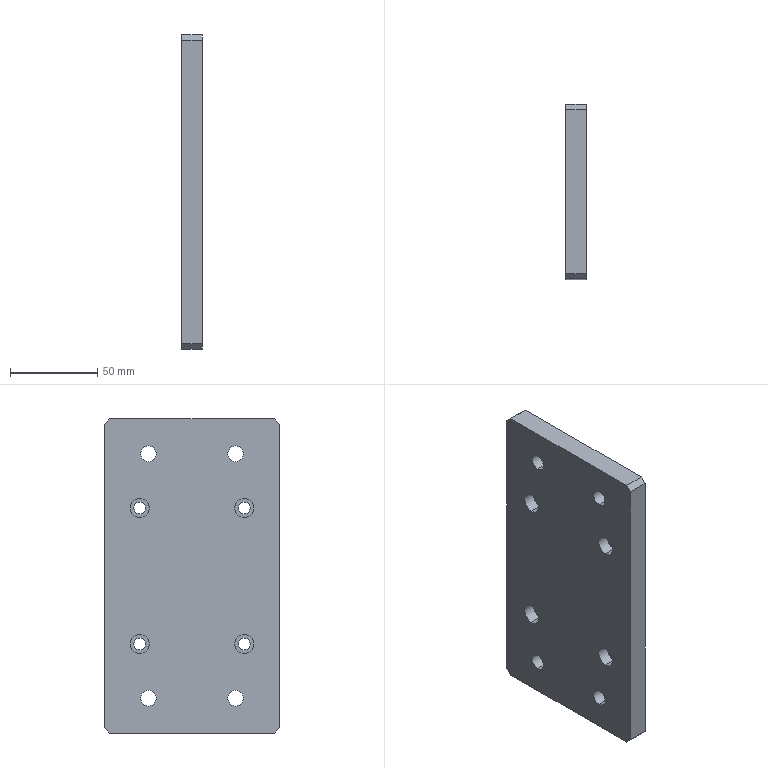Part | SolidWorks | features HoleWzd 2, Chamfer 1, Extrusion 1 | 1 solid | 38 faces | box 12 x 100 x 180 mm | volume 209434 mm3 | cylinder 24 | plane 14 | commonest cylinder face diameters 6.6 x8 9 x8 11 x8
STEP:
#1=CARTESIAN_POINT('',(12.,25.,-74.5));
#2=VERTEX_POINT('',#1);
#3=CARTESIAN_POINT('',(12.,25.,-65.5));
#4=VERTEX_POINT('',#3);
#5=CARTESIAN_POINT('',(12.,25.,-70.));
#6=DIRECTION('',(-1.,0.,0.));
#7=DIRECTION('',(0.,0.,1.));
#8=AXIS2_PLACEMENT_3D('',#5,#6,#7);
#9=CIRCLE('',#8,4.5);
#10=EDGE_CURVE('',#2,#4,#9,.T.);
#11=ORIENTED_EDGE('',*,*,#10,.F.);
#12=CARTESIAN_POINT('',(0.,25.,-74.5));
#13=VERTEX_POINT('',#12);
#14=CARTESIAN_POINT('',(0.,25.,-74.5));
#15=DIRECTION('',(-1.,0.,0.));
#16=VECTOR('',#15,1000.);
#17=LINE('',#14,#16);
#18=EDGE_CURVE('',#2,#13,#17,.T.);
#19=ORIENTED_EDGE('',*,*,#18,.T.);
#20=CARTESIAN_POINT('',(0.,25.,-65.5));
#21=VERTEX_POINT('',#20);
#22=CARTESIAN_POINT('',(0.,25.,-70.));
#23=DIRECTION('',(-1.,0.,0.));
#24=DIRECTION('',(0.,0.,1.));
#25=AXIS2_PLACEMENT_3D('',#22,#23,#24);
#26=CIRCLE('',#25,4.5);
#27=EDGE_CURVE('',#13,#21,#26,.T.);
#28=ORIENTED_EDGE('',*,*,#27,.T.);
#29=CARTESIAN_POINT('',(0.,25.,-65.5));
#30=DIRECTION('',(-1.,0.,0.));
#31=VECTOR('',#30,1000.);
#32=LINE('',#29,#31);
#33=EDGE_CURVE('',#4,#21,#32,.T.);
#34=ORIENTED_EDGE('',*,*,#33,.F.);
#35=EDGE_LOOP('',(#11,#19,#28,#34));
#36=FACE_OUTER_BOUND('',#35,.T.);
#37=CARTESIAN_POINT('',(0.,25.,-70.));
#38=DIRECTION('',(-1.,0.,0.));
#39=DIRECTION('',(0.,0.,1.));
#40=AXIS2_PLACEMENT_3D('',#37,#38,#39);
#41=CYLINDRICAL_SURFACE('',#40,4.5);
#42=ADVANCED_FACE('',(#36),#41,.F.);
#43=CARTESIAN_POINT('',(12.,-25.,-74.5));
#44=VERTEX_POINT('',#43);
#45=CARTESIAN_POINT('',(12.,-25.,-65.5));
#46=VERTEX_POINT('',#45);
#47=CARTESIAN_POINT('',(12.,-25.,-70.));
#48=DIRECTION('',(-1.,0.,0.));
#49=DIRECTION('',(0.,0.,1.));
#50=AXIS2_PLACEMENT_3D('',#47,#48,#49);
#51=CIRCLE('',#50,4.5);
#52=EDGE_CURVE('',#44,#46,#51,.T.);
#53=ORIENTED_EDGE('',*,*,#52,.F.);
#54=CARTESIAN_POINT('',(0.,-25.,-74.5));
#55=VERTEX_POINT('',#54);
#56=CARTESIAN_POINT('',(0.,-25.,-74.5));
#57=DIRECTION('',(-1.,0.,0.));
#58=VECTOR('',#57,1000.);
#59=LINE('',#56,#58);
#60=EDGE_CURVE('',#44,#55,#59,.T.);
#61=ORIENTED_EDGE('',*,*,#60,.T.);
#62=CARTESIAN_POINT('',(0.,-25.,-65.5));
#63=VERTEX_POINT('',#62);
#64=CARTESIAN_POINT('',(0.,-25.,-70.));
#65=DIRECTION('',(-1.,0.,0.));
#66=DIRECTION('',(0.,0.,1.));
#67=AXIS2_PLACEMENT_3D('',#64,#65,#66);
#68=CIRCLE('',#67,4.5);
#69=EDGE_CURVE('',#55,#63,#68,.T.);
#70=ORIENTED_EDGE('',*,*,#69,.T.);
#71=CARTESIAN_POINT('',(0.,-25.,-65.5));
#72=DIRECTION('',(-1.,0.,0.));
#73=VECTOR('',#72,1000.);
#74=LINE('',#71,#73);
#75=EDGE_CURVE('',#46,#63,#74,.T.);
#76=ORIENTED_EDGE('',*,*,#75,.F.);
#77=EDGE_LOOP('',(#53,#61,#70,#76));
#78=FACE_OUTER_BOUND('',#77,.T.);
#79=CARTESIAN_POINT('',(0.,-25.,-70.));
#80=DIRECTION('',(-1.,0.,0.));
#81=DIRECTION('',(0.,0.,1.));
#82=AXIS2_PLACEMENT_3D('',#79,#80,#81);
#83=CYLINDRICAL_SURFACE('',#82,4.5);
#84=ADVANCED_FACE('',(#78),#83,.F.);
#85=CARTESIAN_POINT('',(12.,25.,65.5));
#86=VERTEX_POINT('',#85);
#87=CARTESIAN_POINT('',(12.,25.,74.5));
#88=VERTEX_POINT('',#87);
#89=CARTESIAN_POINT('',(12.,25.,70.));
#90=DIRECTION('',(-1.,0.,0.));
#91=DIRECTION('',(0.,0.,1.));
#92=AXIS2_PLACEMENT_3D('',#89,#90,#91);
#93=CIRCLE('',#92,4.5);
#94=EDGE_CURVE('',#86,#88,#93,.T.);
#95=ORIENTED_EDGE('',*,*,#94,.F.);
#96=CARTESIAN_POINT('',(0.,25.,65.5));
#97=VERTEX_POINT('',#96);
#98=CARTESIAN_POINT('',(0.,25.,65.5));
#99=DIRECTION('',(-1.,0.,0.));
#100=VECTOR('',#99,1000.);
#101=LINE('',#98,#100);
#102=EDGE_CURVE('',#86,#97,#101,.T.);
#103=ORIENTED_EDGE('',*,*,#102,.T.);
#104=CARTESIAN_POINT('',(0.,25.,74.5));
#105=VERTEX_POINT('',#104);
#106=CARTESIAN_POINT('',(0.,25.,70.));
#107=DIRECTION('',(-1.,0.,0.));
#108=DIRECTION('',(0.,0.,1.));
#109=AXIS2_PLACEMENT_3D('',#106,#107,#108);
#110=CIRCLE('',#109,4.5);
#111=EDGE_CURVE('',#97,#105,#110,.T.);
#112=ORIENTED_EDGE('',*,*,#111,.T.);
#113=CARTESIAN_POINT('',(0.,25.,74.5));
#114=DIRECTION('',(-1.,0.,0.));
#115=VECTOR('',#114,1000.);
#116=LINE('',#113,#115);
#117=EDGE_CURVE('',#88,#105,#116,.T.);
#118=ORIENTED_EDGE('',*,*,#117,.F.);
#119=EDGE_LOOP('',(#95,#103,#112,#118));
#120=FACE_OUTER_BOUND('',#119,.T.);
#121=CARTESIAN_POINT('',(0.,25.,70.));
#122=DIRECTION('',(-1.,0.,0.));
#123=DIRECTION('',(0.,0.,1.));
#124=AXIS2_PLACEMENT_3D('',#121,#122,#123);
#125=CYLINDRICAL_SURFACE('',#124,4.5);
#126=ADVANCED_FACE('',(#120),#125,.F.);
#127=CARTESIAN_POINT('',(12.,-25.,65.5));
#128=VERTEX_POINT('',#127);
#129=CARTESIAN_POINT('',(12.,-25.,74.5));
#130=VERTEX_POINT('',#129);
#131=CARTESIAN_POINT('',(12.,-25.,70.));
#132=DIRECTION('',(-1.,0.,0.));
#133=DIRECTION('',(0.,0.,1.));
#134=AXIS2_PLACEMENT_3D('',#131,#132,#133);
#135=CIRCLE('',#134,4.5);
#136=EDGE_CURVE('',#128,#130,#135,.T.);
#137=ORIENTED_EDGE('',*,*,#136,.F.);
#138=CARTESIAN_POINT('',(0.,-25.,65.5));
#139=VERTEX_POINT('',#138);
#140=CARTESIAN_POINT('',(0.,-25.,65.5));
#141=DIRECTION('',(-1.,0.,0.));
#142=VECTOR('',#141,1000.);
#143=LINE('',#140,#142);
#144=EDGE_CURVE('',#128,#139,#143,.T.);
#145=ORIENTED_EDGE('',*,*,#144,.T.);
#146=CARTESIAN_POINT('',(0.,-25.,74.5));
#147=VERTEX_POINT('',#146);
#148=CARTESIAN_POINT('',(0.,-25.,70.));
#149=DIRECTION('',(-1.,0.,0.));
#150=DIRECTION('',(0.,0.,1.));
#151=AXIS2_PLACEMENT_3D('',#148,#149,#150);
#152=CIRCLE('',#151,4.5);
#153=EDGE_CURVE('',#139,#147,#152,.T.);
#154=ORIENTED_EDGE('',*,*,#153,.T.);
#155=CARTESIAN_POINT('',(0.,-25.,74.5));
#156=DIRECTION('',(-1.,0.,0.));
#157=VECTOR('',#156,1000.);
#158=LINE('',#155,#157);
#159=EDGE_CURVE('',#130,#147,#158,.T.);
#160=ORIENTED_EDGE('',*,*,#159,.F.);
#161=EDGE_LOOP('',(#137,#145,#154,#160));
#162=FACE_OUTER_BOUND('',#161,.T.);
#163=CARTESIAN_POINT('',(0.,-25.,70.));
#164=DIRECTION('',(-1.,0.,0.));
#165=DIRECTION('',(0.,0.,1.));
#166=AXIS2_PLACEMENT_3D('',#163,#164,#165);
#167=CYLINDRICAL_SURFACE('',#166,4.5);
#168=ADVANCED_FACE('',(#162),#167,.F.);
#169=CARTESIAN_POINT('',(6.8,30.,-44.5));
#170=VERTEX_POINT('',#169);
#171=CARTESIAN_POINT('',(6.8,30.,-33.5));
#172=VERTEX_POINT('',#171);
#173=CARTESIAN_POINT('',(6.8,30.,-39.));
#174=DIRECTION('',(-1.,0.,0.));
#175=DIRECTION('',(0.,0.,1.));
#176=AXIS2_PLACEMENT_3D('',#173,#174,#175);
#177=CIRCLE('',#176,5.5);
#178=EDGE_CURVE('',#170,#172,#177,.T.);
#179=ORIENTED_EDGE('',*,*,#178,.F.);
#180=CARTESIAN_POINT('',(0.,30.,-44.5));
#181=VERTEX_POINT('',#180);
#182=CARTESIAN_POINT('',(0.,30.,-44.5));
#183=DIRECTION('',(-1.,0.,0.));
#184=VECTOR('',#183,1000.);
#185=LINE('',#182,#184);
#186=EDGE_CURVE('',#170,#181,#185,.T.);
#187=ORIENTED_EDGE('',*,*,#186,.T.);
#188=CARTESIAN_POINT('',(0.,30.,-33.5));
#189=VERTEX_POINT('',#188);
#190=CARTESIAN_POINT('',(0.,30.,-39.));
#191=DIRECTION('',(-1.,0.,0.));
#192=DIRECTION('',(0.,0.,1.));
#193=AXIS2_PLACEMENT_3D('',#190,#191,#192);
#194=CIRCLE('',#193,5.5);
#195=EDGE_CURVE('',#181,#189,#194,.T.);
#196=ORIENTED_EDGE('',*,*,#195,.T.);
#197=CARTESIAN_POINT('',(0.,30.,-33.5));
#198=DIRECTION('',(-1.,0.,0.));
#199=VECTOR('',#198,1000.);
#200=LINE('',#197,#199);
#201=EDGE_CURVE('',#172,#189,#200,.T.);
#202=ORIENTED_EDGE('',*,*,#201,.F.);
#203=EDGE_LOOP('',(#179,#187,#196,#202));
#204=FACE_OUTER_BOUND('',#203,.T.);
#205=CARTESIAN_POINT('',(0.,30.,-39.));
#206=DIRECTION('',(-1.,0.,0.));
#207=DIRECTION('',(0.,0.,1.));
#208=AXIS2_PLACEMENT_3D('',#205,#206,#207);
#209=CYLINDRICAL_SURFACE('',#208,5.5);
#210=ADVANCED_FACE('',(#204),#209,.F.);
#211=CARTESIAN_POINT('',(12.,30.,-42.3));
#212=VERTEX_POINT('',#211);
#213=CARTESIAN_POINT('',(12.,30.,-35.7));
#214=VERTEX_POINT('',#213);
#215=CARTESIAN_POINT('',(12.,30.,-39.));
#216=DIRECTION('',(-1.,0.,0.));
#217=DIRECTION('',(0.,0.,1.));
#218=AXIS2_PLACEMENT_3D('',#215,#216,#217);
#219=CIRCLE('',#218,3.3);
#220=EDGE_CURVE('',#212,#214,#219,.T.);
#221=ORIENTED_EDGE('',*,*,#220,.F.);
#222=CARTESIAN_POINT('',(6.8,30.,-42.3));
#223=VERTEX_POINT('',#222);
#224=CARTESIAN_POINT('',(0.,30.,-42.3));
#225=DIRECTION('',(-1.,0.,0.));
#226=VECTOR('',#225,1000.);
#227=LINE('',#224,#226);
#228=EDGE_CURVE('',#212,#223,#227,.T.);
#229=ORIENTED_EDGE('',*,*,#228,.T.);
#230=CARTESIAN_POINT('',(6.8,30.,-35.7));
#231=VERTEX_POINT('',#230);
#232=CARTESIAN_POINT('',(6.8,30.,-39.));
#233=DIRECTION('',(-1.,0.,0.));
#234=DIRECTION('',(0.,0.,1.));
#235=AXIS2_PLACEMENT_3D('',#232,#233,#234);
#236=CIRCLE('',#235,3.3);
#237=EDGE_CURVE('',#223,#231,#236,.T.);
#238=ORIENTED_EDGE('',*,*,#237,.T.);
#239=CARTESIAN_POINT('',(0.,30.,-35.7));
#240=DIRECTION('',(-1.,0.,0.));
#241=VECTOR('',#240,1000.);
#242=LINE('',#239,#241);
#243=EDGE_CURVE('',#214,#231,#242,.T.);
#244=ORIENTED_EDGE('',*,*,#243,.F.);
#245=EDGE_LOOP('',(#221,#229,#238,#244));
#246=FACE_OUTER_BOUND('',#245,.T.);
#247=CARTESIAN_POINT('',(0.,30.,-39.));
#248=DIRECTION('',(-1.,0.,0.));
#249=DIRECTION('',(0.,0.,1.));
#250=AXIS2_PLACEMENT_3D('',#247,#248,#249);
#251=CYLINDRICAL_SURFACE('',#250,3.3);
#252=ADVANCED_FACE('',(#246),#251,.F.);
#253=CARTESIAN_POINT('',(6.8,-30.,-44.5));
#254=VERTEX_POINT('',#253);
#255=CARTESIAN_POINT('',(6.8,-30.,-33.5));
#256=VERTEX_POINT('',#255);
#257=CARTESIAN_POINT('',(6.8,-30.,-39.));
#258=DIRECTION('',(-1.,0.,0.));
#259=DIRECTION('',(0.,0.,1.));
#260=AXIS2_PLACEMENT_3D('',#257,#258,#259);
#261=CIRCLE('',#260,5.5);
#262=EDGE_CURVE('',#254,#256,#261,.T.);
#263=ORIENTED_EDGE('',*,*,#262,.F.);
#264=CARTESIAN_POINT('',(0.,-30.,-44.5));
#265=VERTEX_POINT('',#264);
#266=CARTESIAN_POINT('',(0.,-30.,-44.5));
#267=DIRECTION('',(-1.,0.,0.));
#268=VECTOR('',#267,1000.);
#269=LINE('',#266,#268);
#270=EDGE_CURVE('',#254,#265,#269,.T.);
#271=ORIENTED_EDGE('',*,*,#270,.T.);
#272=CARTESIAN_POINT('',(0.,-30.,-33.5));
#273=VERTEX_POINT('',#272);
#274=CARTESIAN_POINT('',(0.,-30.,-39.));
#275=DIRECTION('',(-1.,0.,0.));
#276=DIRECTION('',(0.,0.,1.));
#277=AXIS2_PLACEMENT_3D('',#274,#275,#276);
#278=CIRCLE('',#277,5.5);
#279=EDGE_CURVE('',#265,#273,#278,.T.);
#280=ORIENTED_EDGE('',*,*,#279,.T.);
#281=CARTESIAN_POINT('',(0.,-30.,-33.5));
#282=DIRECTION('',(-1.,0.,0.));
#283=VECTOR('',#282,1000.);
#284=LINE('',#281,#283);
#285=EDGE_CURVE('',#256,#273,#284,.T.);
#286=ORIENTED_EDGE('',*,*,#285,.F.);
#287=EDGE_LOOP('',(#263,#271,#280,#286));
#288=FACE_OUTER_BOUND('',#287,.T.);
#289=CARTESIAN_POINT('',(0.,-30.,-39.));
#290=DIRECTION('',(-1.,0.,0.));
#291=DIRECTION('',(0.,0.,1.));
#292=AXIS2_PLACEMENT_3D('',#289,#290,#291);
#293=CYLINDRICAL_SURFACE('',#292,5.5);
#294=ADVANCED_FACE('',(#288),#293,.F.);
#295=CARTESIAN_POINT('',(12.,-30.,-42.3));
#296=VERTEX_POINT('',#295);
#297=CARTESIAN_POINT('',(12.,-30.,-35.7));
#298=VERTEX_POINT('',#297);
#299=CARTESIAN_POINT('',(12.,-30.,-39.));
#300=DIRECTION('',(-1.,0.,0.));
#301=DIRECTION('',(0.,0.,1.));
#302=AXIS2_PLACEMENT_3D('',#299,#300,#301);
#303=CIRCLE('',#302,3.3);
#304=EDGE_CURVE('',#296,#298,#303,.T.);
#305=ORIENTED_EDGE('',*,*,#304,.F.);
#306=CARTESIAN_POINT('',(6.8,-30.,-42.3));
#307=VERTEX_POINT('',#306);
#308=CARTESIAN_POINT('',(0.,-30.,-42.3));
#309=DIRECTION('',(-1.,0.,0.));
#310=VECTOR('',#309,1000.);
#311=LINE('',#308,#310);
#312=EDGE_CURVE('',#296,#307,#311,.T.);
#313=ORIENTED_EDGE('',*,*,#312,.T.);
#314=CARTESIAN_POINT('',(6.8,-30.,-35.7));
#315=VERTEX_POINT('',#314);
#316=CARTESIAN_POINT('',(6.8,-30.,-39.));
#317=DIRECTION('',(-1.,0.,0.));
#318=DIRECTION('',(0.,0.,1.));
#319=AXIS2_PLACEMENT_3D('',#316,#317,#318);
#320=CIRCLE('',#319,3.3);
#321=EDGE_CURVE('',#307,#315,#320,.T.);
#322=ORIENTED_EDGE('',*,*,#321,.T.);
#323=CARTESIAN_POINT('',(0.,-30.,-35.7));
#324=DIRECTION('',(-1.,0.,0.));
#325=VECTOR('',#324,1000.);
#326=LINE('',#323,#325);
#327=EDGE_CURVE('',#298,#315,#326,.T.);
#328=ORIENTED_EDGE('',*,*,#327,.F.);
#329=EDGE_LOOP('',(#305,#313,#322,#328));
#330=FACE_OUTER_BOUND('',#329,.T.);
#331=CARTESIAN_POINT('',(0.,-30.,-39.));
#332=DIRECTION('',(-1.,0.,0.));
#333=DIRECTION('',(0.,0.,1.));
#334=AXIS2_PLACEMENT_3D('',#331,#332,#333);
#335=CYLINDRICAL_SURFACE('',#334,3.3);
#336=ADVANCED_FACE('',(#330),#335,.F.);
#337=CARTESIAN_POINT('',(6.8,30.,33.5));
#338=VERTEX_POINT('',#337);
#339=CARTESIAN_POINT('',(6.8,30.,44.5));
#340=VERTEX_POINT('',#339);
#341=CARTESIAN_POINT('',(6.8,30.,39.));
#342=DIRECTION('',(-1.,0.,0.));
#343=DIRECTION('',(0.,0.,1.));
#344=AXIS2_PLACEMENT_3D('',#341,#342,#343);
#345=CIRCLE('',#344,5.5);
#346=EDGE_CURVE('',#338,#340,#345,.T.);
#347=ORIENTED_EDGE('',*,*,#346,.F.);
#348=CARTESIAN_POINT('',(0.,30.,33.5));
#349=VERTEX_POINT('',#348);
#350=CARTESIAN_POINT('',(0.,30.,33.5));
#351=DIRECTION('',(-1.,0.,0.));
#352=VECTOR('',#351,1000.);
#353=LINE('',#350,#352);
#354=EDGE_CURVE('',#338,#349,#353,.T.);
#355=ORIENTED_EDGE('',*,*,#354,.T.);
#356=CARTESIAN_POINT('',(0.,30.,44.5));
#357=VERTEX_POINT('',#356);
#358=CARTESIAN_POINT('',(0.,30.,39.));
#359=DIRECTION('',(-1.,0.,0.));
#360=DIRECTION('',(0.,0.,1.));
#361=AXIS2_PLACEMENT_3D('',#358,#359,#360);
#362=CIRCLE('',#361,5.5);
#363=EDGE_CURVE('',#349,#357,#362,.T.);
#364=ORIENTED_EDGE('',*,*,#363,.T.);
#365=CARTESIAN_POINT('',(0.,30.,44.5));
#366=DIRECTION('',(-1.,0.,0.));
#367=VECTOR('',#366,1000.);
#368=LINE('',#365,#367);
#369=EDGE_CURVE('',#340,#357,#368,.T.);
#370=ORIENTED_EDGE('',*,*,#369,.F.);
#371=EDGE_LOOP('',(#347,#355,#364,#370));
#372=FACE_OUTER_BOUND('',#371,.T.);
#373=CARTESIAN_POINT('',(0.,30.,39.));
#374=DIRECTION('',(-1.,0.,0.));
#375=DIRECTION('',(0.,0.,1.));
#376=AXIS2_PLACEMENT_3D('',#373,#374,#375);
#377=CYLINDRICAL_SURFACE('',#376,5.5);
#378=ADVANCED_FACE('',(#372),#377,.F.);
#379=CARTESIAN_POINT('',(12.,30.,35.7));
#380=VERTEX_POINT('',#379);
#381=CARTESIAN_POINT('',(12.,30.,42.3));
#382=VERTEX_POINT('',#381);
#383=CARTESIAN_POINT('',(12.,30.,39.));
#384=DIRECTION('',(-1.,0.,0.));
#385=DIRECTION('',(0.,0.,1.));
#386=AXIS2_PLACEMENT_3D('',#383,#384,#385);
#387=CIRCLE('',#386,3.3);
#388=EDGE_CURVE('',#380,#382,#387,.T.);
#389=ORIENTED_EDGE('',*,*,#388,.F.);
#390=CARTESIAN_POINT('',(6.8,30.,35.7));
#391=VERTEX_POINT('',#390);
#392=CARTESIAN_POINT('',(0.,30.,35.7));
#393=DIRECTION('',(-1.,0.,0.));
#394=VECTOR('',#393,1000.);
#395=LINE('',#392,#394);
#396=EDGE_CURVE('',#380,#391,#395,.T.);
#397=ORIENTED_EDGE('',*,*,#396,.T.);
#398=CARTESIAN_POINT('',(6.8,30.,42.3));
#399=VERTEX_POINT('',#398);
#400=CARTESIAN_POINT('',(6.8,30.,39.));
#401=DIRECTION('',(-1.,0.,0.));
#402=DIRECTION('',(0.,0.,1.));
#403=AXIS2_PLACEMENT_3D('',#400,#401,#402);
#404=CIRCLE('',#403,3.3);
#405=EDGE_CURVE('',#391,#399,#404,.T.);
#406=ORIENTED_EDGE('',*,*,#405,.T.);
#407=CARTESIAN_POINT('',(0.,30.,42.3));
#408=DIRECTION('',(-1.,0.,0.));
#409=VECTOR('',#408,1000.);
#410=LINE('',#407,#409);
#411=EDGE_CURVE('',#382,#399,#410,.T.);
#412=ORIENTED_EDGE('',*,*,#411,.F.);
#413=EDGE_LOOP('',(#389,#397,#406,#412));
#414=FACE_OUTER_BOUND('',#413,.T.);
#415=CARTESIAN_POINT('',(0.,30.,39.));
#416=DIRECTION('',(-1.,0.,0.));
#417=DIRECTION('',(0.,0.,1.));
#418=AXIS2_PLACEMENT_3D('',#415,#416,#417);
#419=CYLINDRICAL_SURFACE('',#418,3.3);
#420=ADVANCED_FACE('',(#414),#419,.F.);
#421=CARTESIAN_POINT('',(6.8,-30.,33.5));
#422=VERTEX_POINT('',#421);
#423=CARTESIAN_POINT('',(6.8,-30.,44.5));
#424=VERTEX_POINT('',#423);
#425=CARTESIAN_POINT('',(6.8,-30.,39.));
#426=DIRECTION('',(-1.,0.,0.));
#427=DIRECTION('',(0.,0.,1.));
#428=AXIS2_PLACEMENT_3D('',#425,#426,#427);
#429=CIRCLE('',#428,5.5);
#430=EDGE_CURVE('',#422,#424,#429,.T.);
#431=ORIENTED_EDGE('',*,*,#430,.F.);
#432=CARTESIAN_POINT('',(0.,-30.,33.5));
#433=VERTEX_POINT('',#432);
#434=CARTESIAN_POINT('',(0.,-30.,33.5));
#435=DIRECTION('',(-1.,0.,0.));
#436=VECTOR('',#435,1000.);
#437=LINE('',#434,#436);
#438=EDGE_CURVE('',#422,#433,#437,.T.);
#439=ORIENTED_EDGE('',*,*,#438,.T.);
#440=CARTESIAN_POINT('',(0.,-30.,44.5));
#441=VERTEX_POINT('',#440);
#442=CARTESIAN_POINT('',(0.,-30.,39.));
#443=DIRECTION('',(-1.,0.,0.));
#444=DIRECTION('',(0.,0.,1.));
#445=AXIS2_PLACEMENT_3D('',#442,#443,#444);
#446=CIRCLE('',#445,5.5);
#447=EDGE_CURVE('',#433,#441,#446,.T.);
#448=ORIENTED_EDGE('',*,*,#447,.T.);
#449=CARTESIAN_POINT('',(0.,-30.,44.5));
#450=DIRECTION('',(-1.,0.,0.));
#451=VECTOR('',#450,1000.);
#452=LINE('',#449,#451);
#453=EDGE_CURVE('',#424,#441,#452,.T.);
#454=ORIENTED_EDGE('',*,*,#453,.F.);
#455=EDGE_LOOP('',(#431,#439,#448,#454));
#456=FACE_OUTER_BOUND('',#455,.T.);
#457=CARTESIAN_POINT('',(0.,-30.,39.));
#458=DIRECTION('',(-1.,0.,0.));
#459=DIRECTION('',(0.,0.,1.));
#460=AXIS2_PLACEMENT_3D('',#457,#458,#459);
#461=CYLINDRICAL_SURFACE('',#460,5.5);
#462=ADVANCED_FACE('',(#456),#461,.F.);
#463=CARTESIAN_POINT('',(12.,-30.,35.7));
#464=VERTEX_POINT('',#463);
#465=CARTESIAN_POINT('',(12.,-30.,42.3));
#466=VERTEX_POINT('',#465);
#467=CARTESIAN_POINT('',(12.,-30.,39.));
#468=DIRECTION('',(-1.,0.,0.));
#469=DIRECTION('',(0.,0.,1.));
#470=AXIS2_PLACEMENT_3D('',#467,#468,#469);
#471=CIRCLE('',#470,3.3);
#472=EDGE_CURVE('',#464,#466,#471,.T.);
#473=ORIENTED_EDGE('',*,*,#472,.F.);
#474=CARTESIAN_POINT('',(6.8,-30.,35.7));
#475=VERTEX_POINT('',#474);
#476=CARTESIAN_POINT('',(0.,-30.,35.7));
#477=DIRECTION('',(-1.,0.,0.));
#478=VECTOR('',#477,1000.);
#479=LINE('',#476,#478);
#480=EDGE_CURVE('',#464,#475,#479,.T.);
#481=ORIENTED_EDGE('',*,*,#480,.T.);
#482=CARTESIAN_POINT('',(6.8,-30.,42.3));
#483=VERTEX_POINT('',#482);
#484=CARTESIAN_POINT('',(6.8,-30.,39.));
#485=DIRECTION('',(-1.,0.,0.));
#486=DIRECTION('',(0.,0.,1.));
#487=AXIS2_PLACEMENT_3D('',#484,#485,#486);
#488=CIRCLE('',#487,3.3);
#489=EDGE_CURVE('',#475,#483,#488,.T.);
#490=ORIENTED_EDGE('',*,*,#489,.T.);
#491=CARTESIAN_POINT('',(0.,-30.,42.3));
#492=DIRECTION('',(-1.,0.,0.));
#493=VECTOR('',#492,1000.);
#494=LINE('',#491,#493);
#495=EDGE_CURVE('',#466,#483,#494,.T.);
#496=ORIENTED_EDGE('',*,*,#495,.F.);
#497=EDGE_LOOP('',(#473,#481,#490,#496));
#498=FACE_OUTER_BOUND('',#497,.T.);
#499=CARTESIAN_POINT('',(0.,-30.,39.));
#500=DIRECTION('',(-1.,0.,0.));
#501=DIRECTION('',(0.,0.,1.));
#502=AXIS2_PLACEMENT_3D('',#499,#500,#501);
#503=CYLINDRICAL_SURFACE('',#502,3.3);
#504=ADVANCED_FACE('',(#498),#503,.F.);
#505=CARTESIAN_POINT('',(12.,50.,-87.));
#506=VERTEX_POINT('',#505);
#507=CARTESIAN_POINT('',(12.,50.,87.));
#508=VERTEX_POINT('',#507);
#509=CARTESIAN_POINT('',(12.,50.,90.));
#510=DIRECTION('',(0.,0.,1.));
#511=VECTOR('',#510,1000.);
#512=LINE('',#509,#511);
#513=EDGE_CURVE('',#506,#508,#512,.T.);
#514=ORIENTED_EDGE('',*,*,#513,.T.);
#515=CARTESIAN_POINT('',(12.,47.,90.));
#516=VERTEX_POINT('',#515);
#517=CARTESIAN_POINT('',(12.,68.5,68.5));
#518=DIRECTION('',(0.,-0.7071,0.7071));
#519=VECTOR('',#518,1000.);
#520=LINE('',#517,#519);
#521=EDGE_CURVE('',#508,#516,#520,.T.);
#522=ORIENTED_EDGE('',*,*,#521,.T.);
#523=CARTESIAN_POINT('',(12.,-47.,90.));
#524=VERTEX_POINT('',#523);
#525=CARTESIAN_POINT('',(12.,50.,90.));
#526=DIRECTION('',(0.,-1.,0.));
#527=VECTOR('',#526,1000.);
#528=LINE('',#525,#527);
#529=EDGE_CURVE('',#516,#524,#528,.T.);
#530=ORIENTED_EDGE('',*,*,#529,.T.);
#531=CARTESIAN_POINT('',(12.,-50.,87.));
#532=VERTEX_POINT('',#531);
#533=CARTESIAN_POINT('',(12.,-68.5,68.5));
#534=DIRECTION('',(0.,-0.7071,-0.7071));
#535=VECTOR('',#534,1000.);
#536=LINE('',#533,#535);
#537=EDGE_CURVE('',#524,#532,#536,.T.);
#538=ORIENTED_EDGE('',*,*,#537,.T.);
#539=CARTESIAN_POINT('',(12.,-50.,-87.));
#540=VERTEX_POINT('',#539);
#541=CARTESIAN_POINT('',(12.,-50.,90.));
#542=DIRECTION('',(0.,0.,-1.));
#543=VECTOR('',#542,1000.);
#544=LINE('',#541,#543);
#545=EDGE_CURVE('',#532,#540,#544,.T.);
#546=ORIENTED_EDGE('',*,*,#545,.T.);
#547=CARTESIAN_POINT('',(12.,-47.,-90.));
#548=VERTEX_POINT('',#547);
#549=CARTESIAN_POINT('',(12.,-68.5,-68.5));
#550=DIRECTION('',(0.,0.7071,-0.7071));
#551=VECTOR('',#550,1000.);
#552=LINE('',#549,#551);
#553=EDGE_CURVE('',#540,#548,#552,.T.);
#554=ORIENTED_EDGE('',*,*,#553,.T.);
#555=CARTESIAN_POINT('',(12.,47.,-90.));
#556=VERTEX_POINT('',#555);
#557=CARTESIAN_POINT('',(12.,50.,-90.));
#558=DIRECTION('',(0.,1.,0.));
#559=VECTOR('',#558,1000.);
#560=LINE('',#557,#559);
#561=EDGE_CURVE('',#548,#556,#560,.T.);
#562=ORIENTED_EDGE('',*,*,#561,.T.);
#563=CARTESIAN_POINT('',(12.,68.5,-68.5));
#564=DIRECTION('',(0.,0.7071,0.7071));
#565=VECTOR('',#564,1000.);
#566=LINE('',#563,#565);
#567=EDGE_CURVE('',#556,#506,#566,.T.);
#568=ORIENTED_EDGE('',*,*,#567,.T.);
#569=EDGE_LOOP('',(#514,#522,#530,#538,#546,#554,#562,#568));
#570=FACE_OUTER_BOUND('',#569,.T.);
#571=CARTESIAN_POINT('',(12.,-30.,39.));
#572=DIRECTION('',(-1.,0.,0.));
#573=DIRECTION('',(0.,0.,1.));
#574=AXIS2_PLACEMENT_3D('',#571,#572,#573);
#575=CIRCLE('',#574,3.3);
#576=EDGE_CURVE('',#466,#464,#575,.T.);
#577=ORIENTED_EDGE('',*,*,#576,.T.);
#578=ORIENTED_EDGE('',*,*,#472,.T.);
#579=EDGE_LOOP('',(#577,#578));
#580=FACE_BOUND('',#579,.T.);
#581=CARTESIAN_POINT('',(12.,30.,39.));
#582=DIRECTION('',(-1.,0.,0.));
#583=DIRECTION('',(0.,0.,1.));
#584=AXIS2_PLACEMENT_3D('',#581,#582,#583);
#585=CIRCLE('',#584,3.3);
#586=EDGE_CURVE('',#382,#380,#585,.T.);
#587=ORIENTED_EDGE('',*,*,#586,.T.);
#588=ORIENTED_EDGE('',*,*,#388,.T.);
#589=EDGE_LOOP('',(#587,#588));
#590=FACE_BOUND('',#589,.T.);
#591=CARTESIAN_POINT('',(12.,-30.,-39.));
#592=DIRECTION('',(-1.,0.,0.));
#593=DIRECTION('',(0.,0.,1.));
#594=AXIS2_PLACEMENT_3D('',#591,#592,#593);
#595=CIRCLE('',#594,3.3);
#596=EDGE_CURVE('',#298,#296,#595,.T.);
#597=ORIENTED_EDGE('',*,*,#596,.T.);
#598=ORIENTED_EDGE('',*,*,#304,.T.);
#599=EDGE_LOOP('',(#597,#598));
#600=FACE_BOUND('',#599,.T.);
#601=CARTESIAN_POINT('',(12.,30.,-39.));
#602=DIRECTION('',(-1.,0.,0.));
#603=DIRECTION('',(0.,0.,1.));
#604=AXIS2_PLACEMENT_3D('',#601,#602,#603);
#605=CIRCLE('',#604,3.3);
#606=EDGE_CURVE('',#214,#212,#605,.T.);
#607=ORIENTED_EDGE('',*,*,#606,.T.);
#608=ORIENTED_EDGE('',*,*,#220,.T.);
#609=EDGE_LOOP('',(#607,#608));
#610=FACE_BOUND('',#609,.T.);
#611=CARTESIAN_POINT('',(12.,-25.,70.));
#612=DIRECTION('',(-1.,0.,0.));
#613=DIRECTION('',(0.,0.,1.));
#614=AXIS2_PLACEMENT_3D('',#611,#612,#613);
#615=CIRCLE('',#614,4.5);
#616=EDGE_CURVE('',#130,#128,#615,.T.);
#617=ORIENTED_EDGE('',*,*,#616,.T.);
#618=ORIENTED_EDGE('',*,*,#136,.T.);
#619=EDGE_LOOP('',(#617,#618));
#620=FACE_BOUND('',#619,.T.);
#621=CARTESIAN_POINT('',(12.,25.,70.));
#622=DIRECTION('',(-1.,0.,0.));
#623=DIRECTION('',(0.,0.,1.));
#624=AXIS2_PLACEMENT_3D('',#621,#622,#623);
#625=CIRCLE('',#624,4.5);
#626=EDGE_CURVE('',#88,#86,#625,.T.);
#627=ORIENTED_EDGE('',*,*,#626,.T.);
#628=ORIENTED_EDGE('',*,*,#94,.T.);
#629=EDGE_LOOP('',(#627,#628));
#630=FACE_BOUND('',#629,.T.);
#631=CARTESIAN_POINT('',(12.,-25.,-70.));
#632=DIRECTION('',(-1.,0.,0.));
#633=DIRECTION('',(0.,0.,1.));
#634=AXIS2_PLACEMENT_3D('',#631,#632,#633);
#635=CIRCLE('',#634,4.5);
#636=EDGE_CURVE('',#46,#44,#635,.T.);
#637=ORIENTED_EDGE('',*,*,#636,.T.);
#638=ORIENTED_EDGE('',*,*,#52,.T.);
#639=EDGE_LOOP('',(#637,#638));
#640=FACE_BOUND('',#639,.T.);
#641=CARTESIAN_POINT('',(12.,25.,-70.));
#642=DIRECTION('',(-1.,0.,0.));
#643=DIRECTION('',(0.,0.,1.));
#644=AXIS2_PLACEMENT_3D('',#641,#642,#643);
#645=CIRCLE('',#644,4.5);
#646=EDGE_CURVE('',#4,#2,#645,.T.);
#647=ORIENTED_EDGE('',*,*,#646,.T.);
#648=ORIENTED_EDGE('',*,*,#10,.T.);
#649=EDGE_LOOP('',(#647,#648));
#650=FACE_BOUND('',#649,.T.);
#651=CARTESIAN_POINT('',(12.,0.,0.));
#652=DIRECTION('',(1.,0.,0.));
#653=DIRECTION('',(0.,0.,-1.));
#654=AXIS2_PLACEMENT_3D('',#651,#652,#653);
#655=PLANE('',#654);
#656=ADVANCED_FACE('',(#570,#580,#590,#600,#610,#620,#630,#640,#650),#655,.T.);
#657=CARTESIAN_POINT('',(0.,-47.,-90.));
#658=VERTEX_POINT('',#657);
#659=CARTESIAN_POINT('',(0.,47.,-90.));
#660=VERTEX_POINT('',#659);
#661=CARTESIAN_POINT('',(0.,50.,-90.));
#662=DIRECTION('',(0.,1.,0.));
#663=VECTOR('',#662,1000.);
#664=LINE('',#661,#663);
#665=EDGE_CURVE('',#658,#660,#664,.T.);
#666=ORIENTED_EDGE('',*,*,#665,.T.);
#667=CARTESIAN_POINT('',(12.,47.,-90.));
#668=DIRECTION('',(1.,0.,0.));
#669=VECTOR('',#668,1000.);
#670=LINE('',#667,#669);
#671=EDGE_CURVE('',#660,#556,#670,.T.);
#672=ORIENTED_EDGE('',*,*,#671,.T.);
#673=ORIENTED_EDGE('',*,*,#561,.F.);
#674=CARTESIAN_POINT('',(12.,-47.,-90.));
#675=DIRECTION('',(-1.,0.,0.));
#676=VECTOR('',#675,1000.);
#677=LINE('',#674,#676);
#678=EDGE_CURVE('',#548,#658,#677,.T.);
#679=ORIENTED_EDGE('',*,*,#678,.T.);
#680=EDGE_LOOP('',(#666,#672,#673,#679));
#681=FACE_OUTER_BOUND('',#680,.T.);
#682=CARTESIAN_POINT('',(12.,50.,-90.));
#683=DIRECTION('',(0.,0.,1.));
#684=DIRECTION('',(1.,0.,0.));
#685=AXIS2_PLACEMENT_3D('',#682,#683,#684);
#686=PLANE('',#685);
#687=ADVANCED_FACE('',(#681),#686,.F.);
#688=CARTESIAN_POINT('',(0.,50.,-87.));
#689=VERTEX_POINT('',#688);
#690=CARTESIAN_POINT('',(0.,50.,87.));
#691=VERTEX_POINT('',#690);
#692=CARTESIAN_POINT('',(0.,50.,90.));
#693=DIRECTION('',(0.,0.,1.));
#694=VECTOR('',#693,1000.);
#695=LINE('',#692,#694);
#696=EDGE_CURVE('',#689,#691,#695,.T.);
#697=ORIENTED_EDGE('',*,*,#696,.T.);
#698=CARTESIAN_POINT('',(12.,50.,87.));
#699=DIRECTION('',(1.,0.,0.));
#700=VECTOR('',#699,1000.);
#701=LINE('',#698,#700);
#702=EDGE_CURVE('',#691,#508,#701,.T.);
#703=ORIENTED_EDGE('',*,*,#702,.T.);
#704=ORIENTED_EDGE('',*,*,#513,.F.);
#705=CARTESIAN_POINT('',(12.,50.,-87.));
#706=DIRECTION('',(-1.,0.,0.));
#707=VECTOR('',#706,1000.);
#708=LINE('',#705,#707);
#709=EDGE_CURVE('',#506,#689,#708,.T.);
#710=ORIENTED_EDGE('',*,*,#709,.T.);
#711=EDGE_LOOP('',(#697,#703,#704,#710));
#712=FACE_OUTER_BOUND('',#711,.T.);
#713=CARTESIAN_POINT('',(12.,50.,90.));
#714=DIRECTION('',(0.,-1.,0.));
#715=DIRECTION('',(0.,0.,-1.));
#716=AXIS2_PLACEMENT_3D('',#713,#714,#715);
#717=PLANE('',#716);
#718=ADVANCED_FACE('',(#712),#717,.F.);
#719=ORIENTED_EDGE('',*,*,#529,.F.);
#720=CARTESIAN_POINT('',(0.,47.,90.));
#721=VERTEX_POINT('',#720);
#722=CARTESIAN_POINT('',(12.,47.,90.));
#723=DIRECTION('',(-1.,0.,0.));
#724=VECTOR('',#723,1000.);
#725=LINE('',#722,#724);
#726=EDGE_CURVE('',#516,#721,#725,.T.);
#727=ORIENTED_EDGE('',*,*,#726,.T.);
#728=CARTESIAN_POINT('',(0.,-47.,90.));
#729=VERTEX_POINT('',#728);
#730=CARTESIAN_POINT('',(0.,50.,90.));
#731=DIRECTION('',(0.,-1.,0.));
#732=VECTOR('',#731,1000.);
#733=LINE('',#730,#732);
#734=EDGE_CURVE('',#721,#729,#733,.T.);
#735=ORIENTED_EDGE('',*,*,#734,.T.);
#736=CARTESIAN_POINT('',(12.,-47.,90.));
#737=DIRECTION('',(1.,0.,0.));
#738=VECTOR('',#737,1000.);
#739=LINE('',#736,#738);
#740=EDGE_CURVE('',#729,#524,#739,.T.);
#741=ORIENTED_EDGE('',*,*,#740,.T.);
#742=EDGE_LOOP('',(#719,#727,#735,#741));
#743=FACE_OUTER_BOUND('',#742,.T.);
#744=CARTESIAN_POINT('',(12.,50.,90.));
#745=DIRECTION('',(0.,0.,-1.));
#746=DIRECTION('',(0.,1.,0.));
#747=AXIS2_PLACEMENT_3D('',#744,#745,#746);
#748=PLANE('',#747);
#749=ADVANCED_FACE('',(#743),#748,.F.);
#750=ORIENTED_EDGE('',*,*,#545,.F.);
#751=CARTESIAN_POINT('',(0.,-50.,87.));
#752=VERTEX_POINT('',#751);
#753=CARTESIAN_POINT('',(12.,-50.,87.));
#754=DIRECTION('',(-1.,0.,0.));
#755=VECTOR('',#754,1000.);
#756=LINE('',#753,#755);
#757=EDGE_CURVE('',#532,#752,#756,.T.);
#758=ORIENTED_EDGE('',*,*,#757,.T.);
#759=CARTESIAN_POINT('',(0.,-50.,-87.));
#760=VERTEX_POINT('',#759);
#761=CARTESIAN_POINT('',(0.,-50.,90.));
#762=DIRECTION('',(0.,0.,-1.));
#763=VECTOR('',#762,1000.);
#764=LINE('',#761,#763);
#765=EDGE_CURVE('',#752,#760,#764,.T.);
#766=ORIENTED_EDGE('',*,*,#765,.T.);
#767=CARTESIAN_POINT('',(12.,-50.,-87.));
#768=DIRECTION('',(1.,0.,0.));
#769=VECTOR('',#768,1000.);
#770=LINE('',#767,#769);
#771=EDGE_CURVE('',#760,#540,#770,.T.);
#772=ORIENTED_EDGE('',*,*,#771,.T.);
#773=EDGE_LOOP('',(#750,#758,#766,#772));
#774=FACE_OUTER_BOUND('',#773,.T.);
#775=CARTESIAN_POINT('',(12.,-50.,90.));
#776=DIRECTION('',(0.,1.,0.));
#777=DIRECTION('',(0.,0.,1.));
#778=AXIS2_PLACEMENT_3D('',#775,#776,#777);
#779=PLANE('',#778);
#780=ADVANCED_FACE('',(#774),#779,.F.);
#781=CARTESIAN_POINT('',(0.,25.,-70.));
#782=DIRECTION('',(-1.,0.,0.));
#783=DIRECTION('',(0.,0.,1.));
#784=AXIS2_PLACEMENT_3D('',#781,#782,#783);
#785=CIRCLE('',#784,4.5);
#786=EDGE_CURVE('',#21,#13,#785,.T.);
#787=ORIENTED_EDGE('',*,*,#786,.F.);
#788=ORIENTED_EDGE('',*,*,#27,.F.);
#789=EDGE_LOOP('',(#787,#788));
#790=FACE_BOUND('',#789,.T.);
#791=CARTESIAN_POINT('',(0.,-25.,-70.));
#792=DIRECTION('',(-1.,0.,0.));
#793=DIRECTION('',(0.,0.,1.));
#794=AXIS2_PLACEMENT_3D('',#791,#792,#793);
#795=CIRCLE('',#794,4.5);
#796=EDGE_CURVE('',#63,#55,#795,.T.);
#797=ORIENTED_EDGE('',*,*,#796,.F.);
#798=ORIENTED_EDGE('',*,*,#69,.F.);
#799=EDGE_LOOP('',(#797,#798));
#800=FACE_BOUND('',#799,.T.);
#801=CARTESIAN_POINT('',(0.,25.,70.));
#802=DIRECTION('',(-1.,0.,0.));
#803=DIRECTION('',(0.,0.,1.));
#804=AXIS2_PLACEMENT_3D('',#801,#802,#803);
#805=CIRCLE('',#804,4.5);
#806=EDGE_CURVE('',#105,#97,#805,.T.);
#807=ORIENTED_EDGE('',*,*,#806,.F.);
#808=ORIENTED_EDGE('',*,*,#111,.F.);
#809=EDGE_LOOP('',(#807,#808));
#810=FACE_BOUND('',#809,.T.);
#811=CARTESIAN_POINT('',(0.,-25.,70.));
#812=DIRECTION('',(-1.,0.,0.));
#813=DIRECTION('',(0.,0.,1.));
#814=AXIS2_PLACEMENT_3D('',#811,#812,#813);
#815=CIRCLE('',#814,4.5);
#816=EDGE_CURVE('',#147,#139,#815,.T.);
#817=ORIENTED_EDGE('',*,*,#816,.F.);
#818=ORIENTED_EDGE('',*,*,#153,.F.);
#819=EDGE_LOOP('',(#817,#818));
#820=FACE_BOUND('',#819,.T.);
#821=CARTESIAN_POINT('',(0.,30.,-39.));
#822=DIRECTION('',(-1.,0.,0.));
#823=DIRECTION('',(0.,0.,1.));
#824=AXIS2_PLACEMENT_3D('',#821,#822,#823);
#825=CIRCLE('',#824,5.5);
#826=EDGE_CURVE('',#189,#181,#825,.T.);
#827=ORIENTED_EDGE('',*,*,#826,.F.);
#828=ORIENTED_EDGE('',*,*,#195,.F.);
#829=EDGE_LOOP('',(#827,#828));
#830=FACE_BOUND('',#829,.T.);
#831=CARTESIAN_POINT('',(0.,-30.,-39.));
#832=DIRECTION('',(-1.,0.,0.));
#833=DIRECTION('',(0.,0.,1.));
#834=AXIS2_PLACEMENT_3D('',#831,#832,#833);
#835=CIRCLE('',#834,5.5);
#836=EDGE_CURVE('',#273,#265,#835,.T.);
#837=ORIENTED_EDGE('',*,*,#836,.F.);
#838=ORIENTED_EDGE('',*,*,#279,.F.);
#839=EDGE_LOOP('',(#837,#838));
#840=FACE_BOUND('',#839,.T.);
#841=CARTESIAN_POINT('',(0.,30.,39.));
#842=DIRECTION('',(-1.,0.,0.));
#843=DIRECTION('',(0.,0.,1.));
#844=AXIS2_PLACEMENT_3D('',#841,#842,#843);
#845=CIRCLE('',#844,5.5);
#846=EDGE_CURVE('',#357,#349,#845,.T.);
#847=ORIENTED_EDGE('',*,*,#846,.F.);
#848=ORIENTED_EDGE('',*,*,#363,.F.);
#849=EDGE_LOOP('',(#847,#848));
#850=FACE_BOUND('',#849,.T.);
#851=CARTESIAN_POINT('',(0.,-30.,39.));
#852=DIRECTION('',(-1.,0.,0.));
#853=DIRECTION('',(0.,0.,1.));
#854=AXIS2_PLACEMENT_3D('',#851,#852,#853);
#855=CIRCLE('',#854,5.5);
#856=EDGE_CURVE('',#441,#433,#855,.T.);
#857=ORIENTED_EDGE('',*,*,#856,.F.);
#858=ORIENTED_EDGE('',*,*,#447,.F.);
#859=EDGE_LOOP('',(#857,#858));
#860=FACE_BOUND('',#859,.T.);
#861=ORIENTED_EDGE('',*,*,#734,.F.);
#862=CARTESIAN_POINT('',(0.,47.,90.));
#863=DIRECTION('',(0.,0.7071,-0.7071));
#864=VECTOR('',#863,1000.);
#865=LINE('',#862,#864);
#866=EDGE_CURVE('',#721,#691,#865,.T.);
#867=ORIENTED_EDGE('',*,*,#866,.T.);
#868=ORIENTED_EDGE('',*,*,#696,.F.);
#869=CARTESIAN_POINT('',(0.,50.,-87.));
#870=DIRECTION('',(0.,-0.7071,-0.7071));
#871=VECTOR('',#870,1000.);
#872=LINE('',#869,#871);
#873=EDGE_CURVE('',#689,#660,#872,.T.);
#874=ORIENTED_EDGE('',*,*,#873,.T.);
#875=ORIENTED_EDGE('',*,*,#665,.F.);
#876=CARTESIAN_POINT('',(0.,-47.,-90.));
#877=DIRECTION('',(0.,-0.7071,0.7071));
#878=VECTOR('',#877,1000.);
#879=LINE('',#876,#878);
#880=EDGE_CURVE('',#658,#760,#879,.T.);
#881=ORIENTED_EDGE('',*,*,#880,.T.);
#882=ORIENTED_EDGE('',*,*,#765,.F.);
#883=CARTESIAN_POINT('',(0.,-50.,87.));
#884=DIRECTION('',(0.,0.7071,0.7071));
#885=VECTOR('',#884,1000.);
#886=LINE('',#883,#885);
#887=EDGE_CURVE('',#752,#729,#886,.T.);
#888=ORIENTED_EDGE('',*,*,#887,.T.);
#889=EDGE_LOOP('',(#861,#867,#868,#874,#875,#881,#882,#888));
#890=FACE_OUTER_BOUND('',#889,.T.);
#891=CARTESIAN_POINT('',(0.,0.,0.));
#892=DIRECTION('',(1.,0.,0.));
#893=DIRECTION('',(0.,0.,-1.));
#894=AXIS2_PLACEMENT_3D('',#891,#892,#893);
#895=PLANE('',#894);
#896=ADVANCED_FACE('',(#790,#800,#810,#820,#830,#840,#850,#860,#890),#895,.F.);
#897=ORIENTED_EDGE('',*,*,#480,.F.);
#898=ORIENTED_EDGE('',*,*,#576,.F.);
#899=ORIENTED_EDGE('',*,*,#495,.T.);
#900=CARTESIAN_POINT('',(6.8,-30.,39.));
#901=DIRECTION('',(-1.,0.,0.));
#902=DIRECTION('',(0.,0.,1.));
#903=AXIS2_PLACEMENT_3D('',#900,#901,#902);
#904=CIRCLE('',#903,3.3);
#905=EDGE_CURVE('',#483,#475,#904,.T.);
#906=ORIENTED_EDGE('',*,*,#905,.T.);
#907=EDGE_LOOP('',(#897,#898,#899,#906));
#908=FACE_OUTER_BOUND('',#907,.T.);
#909=CARTESIAN_POINT('',(0.,-30.,39.));
#910=DIRECTION('',(-1.,0.,0.));
#911=DIRECTION('',(0.,0.,1.));
#912=AXIS2_PLACEMENT_3D('',#909,#910,#911);
#913=CYLINDRICAL_SURFACE('',#912,3.3);
#914=ADVANCED_FACE('',(#908),#913,.F.);
#915=ORIENTED_EDGE('',*,*,#905,.F.);
#916=ORIENTED_EDGE('',*,*,#489,.F.);
#917=EDGE_LOOP('',(#915,#916));
#918=FACE_BOUND('',#917,.T.);
#919=CARTESIAN_POINT('',(6.8,-30.,39.));
#920=DIRECTION('',(-1.,0.,0.));
#921=DIRECTION('',(0.,0.,1.));
#922=AXIS2_PLACEMENT_3D('',#919,#920,#921);
#923=CIRCLE('',#922,5.5);
#924=EDGE_CURVE('',#424,#422,#923,.T.);
#925=ORIENTED_EDGE('',*,*,#924,.T.);
#926=ORIENTED_EDGE('',*,*,#430,.T.);
#927=EDGE_LOOP('',(#925,#926));
#928=FACE_OUTER_BOUND('',#927,.T.);
#929=CARTESIAN_POINT('',(6.8,-26.7,39.));
#930=DIRECTION('',(1.,0.,0.));
#931=DIRECTION('',(0.,0.,-1.));
#932=AXIS2_PLACEMENT_3D('',#929,#930,#931);
#933=PLANE('',#932);
#934=ADVANCED_FACE('',(#918,#928),#933,.F.);
#935=ORIENTED_EDGE('',*,*,#438,.F.);
#936=ORIENTED_EDGE('',*,*,#924,.F.);
#937=ORIENTED_EDGE('',*,*,#453,.T.);
#938=ORIENTED_EDGE('',*,*,#856,.T.);
#939=EDGE_LOOP('',(#935,#936,#937,#938));
#940=FACE_OUTER_BOUND('',#939,.T.);
#941=CARTESIAN_POINT('',(0.,-30.,39.));
#942=DIRECTION('',(-1.,0.,0.));
#943=DIRECTION('',(0.,0.,1.));
#944=AXIS2_PLACEMENT_3D('',#941,#942,#943);
#945=CYLINDRICAL_SURFACE('',#944,5.5);
#946=ADVANCED_FACE('',(#940),#945,.F.);
#947=ORIENTED_EDGE('',*,*,#396,.F.);
#948=ORIENTED_EDGE('',*,*,#586,.F.);
#949=ORIENTED_EDGE('',*,*,#411,.T.);
#950=CARTESIAN_POINT('',(6.8,30.,39.));
#951=DIRECTION('',(-1.,0.,0.));
#952=DIRECTION('',(0.,0.,1.));
#953=AXIS2_PLACEMENT_3D('',#950,#951,#952);
#954=CIRCLE('',#953,3.3);
#955=EDGE_CURVE('',#399,#391,#954,.T.);
#956=ORIENTED_EDGE('',*,*,#955,.T.);
#957=EDGE_LOOP('',(#947,#948,#949,#956));
#958=FACE_OUTER_BOUND('',#957,.T.);
#959=CARTESIAN_POINT('',(0.,30.,39.));
#960=DIRECTION('',(-1.,0.,0.));
#961=DIRECTION('',(0.,0.,1.));
#962=AXIS2_PLACEMENT_3D('',#959,#960,#961);
#963=CYLINDRICAL_SURFACE('',#962,3.3);
#964=ADVANCED_FACE('',(#958),#963,.F.);
#965=ORIENTED_EDGE('',*,*,#955,.F.);
#966=ORIENTED_EDGE('',*,*,#405,.F.);
#967=EDGE_LOOP('',(#965,#966));
#968=FACE_BOUND('',#967,.T.);
#969=CARTESIAN_POINT('',(6.8,30.,39.));
#970=DIRECTION('',(-1.,0.,0.));
#971=DIRECTION('',(0.,0.,1.));
#972=AXIS2_PLACEMENT_3D('',#969,#970,#971);
#973=CIRCLE('',#972,5.5);
#974=EDGE_CURVE('',#340,#338,#973,.T.);
#975=ORIENTED_EDGE('',*,*,#974,.T.);
#976=ORIENTED_EDGE('',*,*,#346,.T.);
#977=EDGE_LOOP('',(#975,#976));
#978=FACE_OUTER_BOUND('',#977,.T.);
#979=CARTESIAN_POINT('',(6.8,33.3,39.));
#980=DIRECTION('',(1.,0.,0.));
#981=DIRECTION('',(0.,0.,-1.));
#982=AXIS2_PLACEMENT_3D('',#979,#980,#981);
#983=PLANE('',#982);
#984=ADVANCED_FACE('',(#968,#978),#983,.F.);
#985=ORIENTED_EDGE('',*,*,#354,.F.);
#986=ORIENTED_EDGE('',*,*,#974,.F.);
#987=ORIENTED_EDGE('',*,*,#369,.T.);
#988=ORIENTED_EDGE('',*,*,#846,.T.);
#989=EDGE_LOOP('',(#985,#986,#987,#988));
#990=FACE_OUTER_BOUND('',#989,.T.);
#991=CARTESIAN_POINT('',(0.,30.,39.));
#992=DIRECTION('',(-1.,0.,0.));
#993=DIRECTION('',(0.,0.,1.));
#994=AXIS2_PLACEMENT_3D('',#991,#992,#993);
#995=CYLINDRICAL_SURFACE('',#994,5.5);
#996=ADVANCED_FACE('',(#990),#995,.F.);
#997=ORIENTED_EDGE('',*,*,#312,.F.);
#998=ORIENTED_EDGE('',*,*,#596,.F.);
#999=ORIENTED_EDGE('',*,*,#327,.T.);
#1000=CARTESIAN_POINT('',(6.8,-30.,-39.));
#1001=DIRECTION('',(-1.,0.,0.));
#1002=DIRECTION('',(0.,0.,1.));
#1003=AXIS2_PLACEMENT_3D('',#1000,#1001,#1002);
#1004=CIRCLE('',#1003,3.3);
#1005=EDGE_CURVE('',#315,#307,#1004,.T.);
#1006=ORIENTED_EDGE('',*,*,#1005,.T.);
#1007=EDGE_LOOP('',(#997,#998,#999,#1006));
#1008=FACE_OUTER_BOUND('',#1007,.T.);
#1009=CARTESIAN_POINT('',(0.,-30.,-39.));
#1010=DIRECTION('',(-1.,0.,0.));
#1011=DIRECTION('',(0.,0.,1.));
#1012=AXIS2_PLACEMENT_3D('',#1009,#1010,#1011);
#1013=CYLINDRICAL_SURFACE('',#1012,3.3);
#1014=ADVANCED_FACE('',(#1008),#1013,.F.);
#1015=ORIENTED_EDGE('',*,*,#1005,.F.);
#1016=ORIENTED_EDGE('',*,*,#321,.F.);
#1017=EDGE_LOOP('',(#1015,#1016));
#1018=FACE_BOUND('',#1017,.T.);
#1019=CARTESIAN_POINT('',(6.8,-30.,-39.));
#1020=DIRECTION('',(-1.,0.,0.));
#1021=DIRECTION('',(0.,0.,1.));
#1022=AXIS2_PLACEMENT_3D('',#1019,#1020,#1021);
#1023=CIRCLE('',#1022,5.5);
#1024=EDGE_CURVE('',#256,#254,#1023,.T.);
#1025=ORIENTED_EDGE('',*,*,#1024,.T.);
#1026=ORIENTED_EDGE('',*,*,#262,.T.);
#1027=EDGE_LOOP('',(#1025,#1026));
#1028=FACE_OUTER_BOUND('',#1027,.T.);
#1029=CARTESIAN_POINT('',(6.8,-26.7,-39.));
#1030=DIRECTION('',(1.,0.,0.));
#1031=DIRECTION('',(0.,0.,-1.));
#1032=AXIS2_PLACEMENT_3D('',#1029,#1030,#1031);
#1033=PLANE('',#1032);
#1034=ADVANCED_FACE('',(#1018,#1028),#1033,.F.);
#1035=ORIENTED_EDGE('',*,*,#270,.F.);
#1036=ORIENTED_EDGE('',*,*,#1024,.F.);
#1037=ORIENTED_EDGE('',*,*,#285,.T.);
#1038=ORIENTED_EDGE('',*,*,#836,.T.);
#1039=EDGE_LOOP('',(#1035,#1036,#1037,#1038));
#1040=FACE_OUTER_BOUND('',#1039,.T.);
#1041=CARTESIAN_POINT('',(0.,-30.,-39.));
#1042=DIRECTION('',(-1.,0.,0.));
#1043=DIRECTION('',(0.,0.,1.));
#1044=AXIS2_PLACEMENT_3D('',#1041,#1042,#1043);
#1045=CYLINDRICAL_SURFACE('',#1044,5.5);
#1046=ADVANCED_FACE('',(#1040),#1045,.F.);
#1047=ORIENTED_EDGE('',*,*,#228,.F.);
#1048=ORIENTED_EDGE('',*,*,#606,.F.);
#1049=ORIENTED_EDGE('',*,*,#243,.T.);
#1050=CARTESIAN_POINT('',(6.8,30.,-39.));
#1051=DIRECTION('',(-1.,0.,0.));
#1052=DIRECTION('',(0.,0.,1.));
#1053=AXIS2_PLACEMENT_3D('',#1050,#1051,#1052);
#1054=CIRCLE('',#1053,3.3);
#1055=EDGE_CURVE('',#231,#223,#1054,.T.);
#1056=ORIENTED_EDGE('',*,*,#1055,.T.);
#1057=EDGE_LOOP('',(#1047,#1048,#1049,#1056));
#1058=FACE_OUTER_BOUND('',#1057,.T.);
#1059=CARTESIAN_POINT('',(0.,30.,-39.));
#1060=DIRECTION('',(-1.,0.,0.));
#1061=DIRECTION('',(0.,0.,1.));
#1062=AXIS2_PLACEMENT_3D('',#1059,#1060,#1061);
#1063=CYLINDRICAL_SURFACE('',#1062,3.3);
#1064=ADVANCED_FACE('',(#1058),#1063,.F.);
#1065=ORIENTED_EDGE('',*,*,#1055,.F.);
#1066=ORIENTED_EDGE('',*,*,#237,.F.);
#1067=EDGE_LOOP('',(#1065,#1066));
#1068=FACE_BOUND('',#1067,.T.);
#1069=CARTESIAN_POINT('',(6.8,30.,-39.));
#1070=DIRECTION('',(-1.,0.,0.));
#1071=DIRECTION('',(0.,0.,1.));
#1072=AXIS2_PLACEMENT_3D('',#1069,#1070,#1071);
#1073=CIRCLE('',#1072,5.5);
#1074=EDGE_CURVE('',#172,#170,#1073,.T.);
#1075=ORIENTED_EDGE('',*,*,#1074,.T.);
#1076=ORIENTED_EDGE('',*,*,#178,.T.);
#1077=EDGE_LOOP('',(#1075,#1076));
#1078=FACE_OUTER_BOUND('',#1077,.T.);
#1079=CARTESIAN_POINT('',(6.8,33.3,-39.));
#1080=DIRECTION('',(1.,0.,0.));
#1081=DIRECTION('',(0.,0.,-1.));
#1082=AXIS2_PLACEMENT_3D('',#1079,#1080,#1081);
#1083=PLANE('',#1082);
#1084=ADVANCED_FACE('',(#1068,#1078),#1083,.F.);
#1085=ORIENTED_EDGE('',*,*,#186,.F.);
#1086=ORIENTED_EDGE('',*,*,#1074,.F.);
#1087=ORIENTED_EDGE('',*,*,#201,.T.);
#1088=ORIENTED_EDGE('',*,*,#826,.T.);
#1089=EDGE_LOOP('',(#1085,#1086,#1087,#1088));
#1090=FACE_OUTER_BOUND('',#1089,.T.);
#1091=CARTESIAN_POINT('',(0.,30.,-39.));
#1092=DIRECTION('',(-1.,0.,0.));
#1093=DIRECTION('',(0.,0.,1.));
#1094=AXIS2_PLACEMENT_3D('',#1091,#1092,#1093);
#1095=CYLINDRICAL_SURFACE('',#1094,5.5);
#1096=ADVANCED_FACE('',(#1090),#1095,.F.);
#1097=ORIENTED_EDGE('',*,*,#144,.F.);
#1098=ORIENTED_EDGE('',*,*,#616,.F.);
#1099=ORIENTED_EDGE('',*,*,#159,.T.);
#1100=ORIENTED_EDGE('',*,*,#816,.T.);
#1101=EDGE_LOOP('',(#1097,#1098,#1099,#1100));
#1102=FACE_OUTER_BOUND('',#1101,.T.);
#1103=CARTESIAN_POINT('',(0.,-25.,70.));
#1104=DIRECTION('',(-1.,0.,0.));
#1105=DIRECTION('',(0.,0.,1.));
#1106=AXIS2_PLACEMENT_3D('',#1103,#1104,#1105);
#1107=CYLINDRICAL_SURFACE('',#1106,4.5);
#1108=ADVANCED_FACE('',(#1102),#1107,.F.);
#1109=ORIENTED_EDGE('',*,*,#102,.F.);
#1110=ORIENTED_EDGE('',*,*,#626,.F.);
#1111=ORIENTED_EDGE('',*,*,#117,.T.);
#1112=ORIENTED_EDGE('',*,*,#806,.T.);
#1113=EDGE_LOOP('',(#1109,#1110,#1111,#1112));
#1114=FACE_OUTER_BOUND('',#1113,.T.);
#1115=CARTESIAN_POINT('',(0.,25.,70.));
#1116=DIRECTION('',(-1.,0.,0.));
#1117=DIRECTION('',(0.,0.,1.));
#1118=AXIS2_PLACEMENT_3D('',#1115,#1116,#1117);
#1119=CYLINDRICAL_SURFACE('',#1118,4.5);
#1120=ADVANCED_FACE('',(#1114),#1119,.F.);
#1121=ORIENTED_EDGE('',*,*,#60,.F.);
#1122=ORIENTED_EDGE('',*,*,#636,.F.);
#1123=ORIENTED_EDGE('',*,*,#75,.T.);
#1124=ORIENTED_EDGE('',*,*,#796,.T.);
#1125=EDGE_LOOP('',(#1121,#1122,#1123,#1124));
#1126=FACE_OUTER_BOUND('',#1125,.T.);
#1127=CARTESIAN_POINT('',(0.,-25.,-70.));
#1128=DIRECTION('',(-1.,0.,0.));
#1129=DIRECTION('',(0.,0.,1.));
#1130=AXIS2_PLACEMENT_3D('',#1127,#1128,#1129);
#1131=CYLINDRICAL_SURFACE('',#1130,4.5);
#1132=ADVANCED_FACE('',(#1126),#1131,.F.);
#1133=ORIENTED_EDGE('',*,*,#18,.F.);
#1134=ORIENTED_EDGE('',*,*,#646,.F.);
#1135=ORIENTED_EDGE('',*,*,#33,.T.);
#1136=ORIENTED_EDGE('',*,*,#786,.T.);
#1137=EDGE_LOOP('',(#1133,#1134,#1135,#1136));
#1138=FACE_OUTER_BOUND('',#1137,.T.);
#1139=CARTESIAN_POINT('',(0.,25.,-70.));
#1140=DIRECTION('',(-1.,0.,0.));
#1141=DIRECTION('',(0.,0.,1.));
#1142=AXIS2_PLACEMENT_3D('',#1139,#1140,#1141);
#1143=CYLINDRICAL_SURFACE('',#1142,4.5);
#1144=ADVANCED_FACE('',(#1138),#1143,.F.);
#1145=ORIENTED_EDGE('',*,*,#521,.F.);
#1146=ORIENTED_EDGE('',*,*,#702,.F.);
#1147=ORIENTED_EDGE('',*,*,#866,.F.);
#1148=ORIENTED_EDGE('',*,*,#726,.F.);
#1149=EDGE_LOOP('',(#1145,#1146,#1147,#1148));
#1150=FACE_OUTER_BOUND('',#1149,.T.);
#1151=CARTESIAN_POINT('',(12.,47.,90.));
#1152=DIRECTION('',(0.,-0.7071,-0.7071));
#1153=DIRECTION('',(-1.,0.,0.));
#1154=AXIS2_PLACEMENT_3D('',#1151,#1152,#1153);
#1155=PLANE('',#1154);
#1156=ADVANCED_FACE('',(#1150),#1155,.F.);
#1157=ORIENTED_EDGE('',*,*,#537,.F.);
#1158=ORIENTED_EDGE('',*,*,#740,.F.);
#1159=ORIENTED_EDGE('',*,*,#887,.F.);
#1160=ORIENTED_EDGE('',*,*,#757,.F.);
#1161=EDGE_LOOP('',(#1157,#1158,#1159,#1160));
#1162=FACE_OUTER_BOUND('',#1161,.T.);
#1163=CARTESIAN_POINT('',(12.,-50.,87.));
#1164=DIRECTION('',(0.,0.7071,-0.7071));
#1165=DIRECTION('',(-1.,0.,0.));
#1166=AXIS2_PLACEMENT_3D('',#1163,#1164,#1165);
#1167=PLANE('',#1166);
#1168=ADVANCED_FACE('',(#1162),#1167,.F.);
#1169=ORIENTED_EDGE('',*,*,#567,.F.);
#1170=ORIENTED_EDGE('',*,*,#671,.F.);
#1171=ORIENTED_EDGE('',*,*,#873,.F.);
#1172=ORIENTED_EDGE('',*,*,#709,.F.);
#1173=EDGE_LOOP('',(#1169,#1170,#1171,#1172));
#1174=FACE_OUTER_BOUND('',#1173,.T.);
#1175=CARTESIAN_POINT('',(12.,50.,-87.));
#1176=DIRECTION('',(0.,-0.7071,0.7071));
#1177=DIRECTION('',(-1.,0.,0.));
#1178=AXIS2_PLACEMENT_3D('',#1175,#1176,#1177);
#1179=PLANE('',#1178);
#1180=ADVANCED_FACE('',(#1174),#1179,.F.);
#1181=ORIENTED_EDGE('',*,*,#553,.F.);
#1182=ORIENTED_EDGE('',*,*,#771,.F.);
#1183=ORIENTED_EDGE('',*,*,#880,.F.);
#1184=ORIENTED_EDGE('',*,*,#678,.F.);
#1185=EDGE_LOOP('',(#1181,#1182,#1183,#1184));
#1186=FACE_OUTER_BOUND('',#1185,.T.);
#1187=CARTESIAN_POINT('',(12.,-47.,-90.));
#1188=DIRECTION('',(0.,0.7071,0.7071));
#1189=DIRECTION('',(-1.,0.,0.));
#1190=AXIS2_PLACEMENT_3D('',#1187,#1188,#1189);
#1191=PLANE('',#1190);
#1192=ADVANCED_FACE('',(#1186),#1191,.F.);
#1193=CLOSED_SHELL('',(#42,#84,#126,#168,#210,#252,#294,#336,#378,#420,#462,#504,#656,#687,#718,#749,#780,#896,#914,#934,#946,#964,#984,#996,#1014,#1034,#1046,#1064,#1084,#1096,#1108,#1120,#1132,#1144,#1156,#1168,#1180,#1192));
#1194=MANIFOLD_SOLID_BREP('',#1193);
#1195=CARTESIAN_POINT('',(0.,0.,0.));
#1196=DIRECTION('',(0.,0.,1.));
#1197=DIRECTION('',(1.,0.,0.));
#1198=AXIS2_PLACEMENT_3D('',#1195,#1196,#1197);
#1199=(LENGTH_UNIT()NAMED_UNIT(*)SI_UNIT(.MILLI.,.METRE.));
#1200=UNCERTAINTY_MEASURE_WITH_UNIT(LENGTH_MEASURE(0.00001),#1199,'','');
#1201=(NAMED_UNIT(*)PLANE_ANGLE_UNIT()SI_UNIT($,.RADIAN.));
#1202=(NAMED_UNIT(*)SI_UNIT($,.STERADIAN.)SOLID_ANGLE_UNIT());
#1203=(GEOMETRIC_REPRESENTATION_CONTEXT(3)GLOBAL_UNCERTAINTY_ASSIGNED_CONTEXT((#1200))GLOBAL_UNIT_ASSIGNED_CONTEXT((#1199,#1201,#1202))REPRESENTATION_CONTEXT('',''));
#1204=ADVANCED_BREP_SHAPE_REPRESENTATION('',(#1194,#1198),#1203);